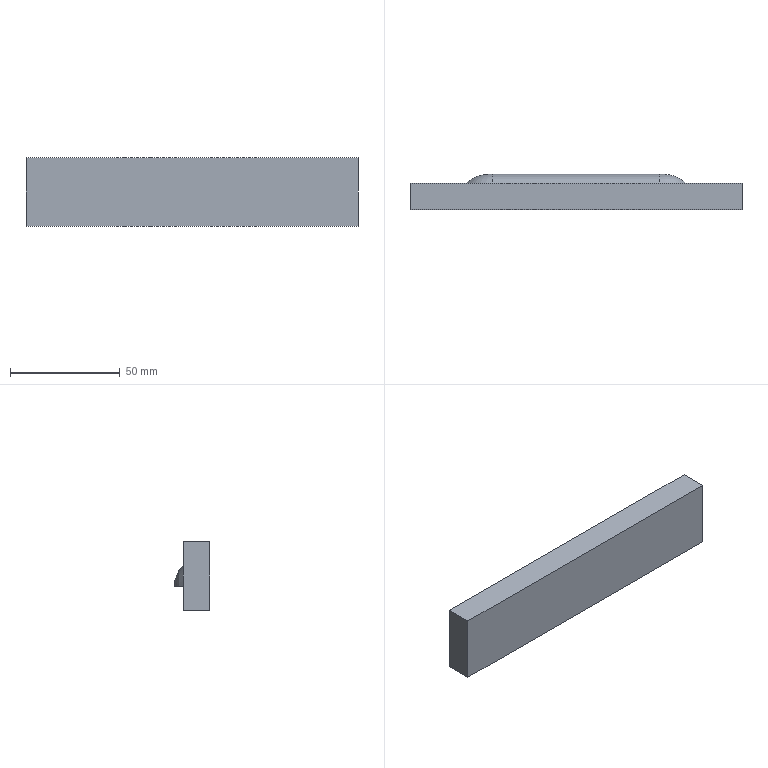Part | SolidWorks | features Fillet 2, Extrusion 1, FormToolCreator 1, ICE 1 | 1 solid | 10 faces | box 151.025 x 16 x 31.377 mm | volume 59353 mm3 | plane 7 | torus 2 | cylinder 1 | commonest cylinder face diameters 29 x1
STEP:
#1=CARTESIAN_POINT('',(75.513,12.,15.689));
#2=VERTEX_POINT('',#1);
#3=CARTESIAN_POINT('',(75.513,12.,-15.689));
#4=VERTEX_POINT('',#3);
#5=CARTESIAN_POINT('',(75.513,12.,-15.689));
#6=DIRECTION('',(0.,0.,-1.));
#7=VECTOR('',#6,1000.);
#8=LINE('',#5,#7);
#9=EDGE_CURVE('',#2,#4,#8,.T.);
#10=ORIENTED_EDGE('',*,*,#9,.T.);
#11=CARTESIAN_POINT('',(-75.513,12.,-15.689));
#12=VERTEX_POINT('',#11);
#13=CARTESIAN_POINT('',(-75.513,12.,-15.689));
#14=DIRECTION('',(-1.,0.,0.));
#15=VECTOR('',#14,1000.);
#16=LINE('',#13,#15);
#17=EDGE_CURVE('',#4,#12,#16,.T.);
#18=ORIENTED_EDGE('',*,*,#17,.T.);
#19=CARTESIAN_POINT('',(-75.513,12.,15.689));
#20=VERTEX_POINT('',#19);
#21=CARTESIAN_POINT('',(-75.513,12.,-15.689));
#22=DIRECTION('',(0.,0.,1.));
#23=VECTOR('',#22,1000.);
#24=LINE('',#21,#23);
#25=EDGE_CURVE('',#12,#20,#24,.T.);
#26=ORIENTED_EDGE('',*,*,#25,.T.);
#27=CARTESIAN_POINT('',(-75.513,12.,15.689));
#28=DIRECTION('',(1.,0.,0.));
#29=VECTOR('',#28,1000.);
#30=LINE('',#27,#29);
#31=EDGE_CURVE('',#20,#2,#30,.T.);
#32=ORIENTED_EDGE('',*,*,#31,.T.);
#33=EDGE_LOOP('',(#10,#18,#26,#32));
#34=FACE_OUTER_BOUND('',#33,.T.);
#35=CARTESIAN_POINT('',(50.,12.,-5.));
#36=VERTEX_POINT('',#35);
#37=CARTESIAN_POINT('',(-50.,12.,-5.));
#38=VERTEX_POINT('',#37);
#39=CARTESIAN_POINT('',(-50.,12.,-5.));
#40=DIRECTION('',(-1.,0.,0.));
#41=VECTOR('',#40,1000.);
#42=LINE('',#39,#41);
#43=EDGE_CURVE('',#36,#38,#42,.T.);
#44=ORIENTED_EDGE('',*,*,#43,.F.);
#45=CARTESIAN_POINT('',(38.168,12.,5.));
#46=VERTEX_POINT('',#45);
#47=CARTESIAN_POINT('',(38.168,12.,-7.));
#48=DIRECTION('',(0.,-1.,0.));
#49=DIRECTION('',(0.,0.,1.));
#50=AXIS2_PLACEMENT_3D('',#47,#48,#49);
#51=CIRCLE('',#50,12.);
#52=EDGE_CURVE('',#36,#46,#51,.T.);
#53=ORIENTED_EDGE('',*,*,#52,.T.);
#54=CARTESIAN_POINT('',(-38.168,12.,5.));
#55=VERTEX_POINT('',#54);
#56=CARTESIAN_POINT('',(-50.,12.,5.));
#57=DIRECTION('',(1.,0.,0.));
#58=VECTOR('',#57,1000.);
#59=LINE('',#56,#58);
#60=EDGE_CURVE('',#55,#46,#59,.T.);
#61=ORIENTED_EDGE('',*,*,#60,.F.);
#62=CARTESIAN_POINT('',(-38.168,12.,-7.));
#63=DIRECTION('',(0.,-1.,0.));
#64=DIRECTION('',(0.,0.,1.));
#65=AXIS2_PLACEMENT_3D('',#62,#63,#64);
#66=CIRCLE('',#65,12.);
#67=EDGE_CURVE('',#55,#38,#66,.T.);
#68=ORIENTED_EDGE('',*,*,#67,.T.);
#69=EDGE_LOOP('',(#44,#53,#61,#68));
#70=FACE_BOUND('',#69,.T.);
#71=CARTESIAN_POINT('',(0.,12.,0.));
#72=DIRECTION('',(0.,1.,0.));
#73=DIRECTION('',(0.,0.,1.));
#74=AXIS2_PLACEMENT_3D('',#71,#72,#73);
#75=PLANE('',#74);
#76=ADVANCED_FACE('',(#34,#70),#75,.T.);
#77=CARTESIAN_POINT('',(75.513,0.,15.689));
#78=VERTEX_POINT('',#77);
#79=CARTESIAN_POINT('',(75.513,0.,-15.689));
#80=VERTEX_POINT('',#79);
#81=CARTESIAN_POINT('',(75.513,0.,-15.689));
#82=DIRECTION('',(0.,0.,-1.));
#83=VECTOR('',#82,1000.);
#84=LINE('',#81,#83);
#85=EDGE_CURVE('',#78,#80,#84,.T.);
#86=ORIENTED_EDGE('',*,*,#85,.T.);
#87=CARTESIAN_POINT('',(75.513,12.,-15.689));
#88=DIRECTION('',(0.,-1.,0.));
#89=VECTOR('',#88,1000.);
#90=LINE('',#87,#89);
#91=EDGE_CURVE('',#4,#80,#90,.T.);
#92=ORIENTED_EDGE('',*,*,#91,.F.);
#93=ORIENTED_EDGE('',*,*,#9,.F.);
#94=CARTESIAN_POINT('',(75.513,12.,15.689));
#95=DIRECTION('',(0.,-1.,0.));
#96=VECTOR('',#95,1000.);
#97=LINE('',#94,#96);
#98=EDGE_CURVE('',#2,#78,#97,.T.);
#99=ORIENTED_EDGE('',*,*,#98,.T.);
#100=EDGE_LOOP('',(#86,#92,#93,#99));
#101=FACE_OUTER_BOUND('',#100,.T.);
#102=CARTESIAN_POINT('',(75.513,12.,-15.689));
#103=DIRECTION('',(-1.,0.,0.));
#104=DIRECTION('',(0.,0.,1.));
#105=AXIS2_PLACEMENT_3D('',#102,#103,#104);
#106=PLANE('',#105);
#107=ADVANCED_FACE('',(#101),#106,.F.);
#108=CARTESIAN_POINT('',(-75.513,0.,-15.689));
#109=VERTEX_POINT('',#108);
#110=CARTESIAN_POINT('',(-75.513,0.,-15.689));
#111=DIRECTION('',(-1.,0.,0.));
#112=VECTOR('',#111,1000.);
#113=LINE('',#110,#112);
#114=EDGE_CURVE('',#80,#109,#113,.T.);
#115=ORIENTED_EDGE('',*,*,#114,.T.);
#116=CARTESIAN_POINT('',(-75.513,12.,-15.689));
#117=DIRECTION('',(0.,-1.,0.));
#118=VECTOR('',#117,1000.);
#119=LINE('',#116,#118);
#120=EDGE_CURVE('',#12,#109,#119,.T.);
#121=ORIENTED_EDGE('',*,*,#120,.F.);
#122=ORIENTED_EDGE('',*,*,#17,.F.);
#123=ORIENTED_EDGE('',*,*,#91,.T.);
#124=EDGE_LOOP('',(#115,#121,#122,#123));
#125=FACE_OUTER_BOUND('',#124,.T.);
#126=CARTESIAN_POINT('',(-75.513,12.,-15.689));
#127=DIRECTION('',(0.,0.,1.));
#128=DIRECTION('',(1.,0.,0.));
#129=AXIS2_PLACEMENT_3D('',#126,#127,#128);
#130=PLANE('',#129);
#131=ADVANCED_FACE('',(#125),#130,.F.);
#132=CARTESIAN_POINT('',(-75.513,0.,15.689));
#133=VERTEX_POINT('',#132);
#134=CARTESIAN_POINT('',(-75.513,0.,-15.689));
#135=DIRECTION('',(0.,0.,1.));
#136=VECTOR('',#135,1000.);
#137=LINE('',#134,#136);
#138=EDGE_CURVE('',#109,#133,#137,.T.);
#139=ORIENTED_EDGE('',*,*,#138,.T.);
#140=CARTESIAN_POINT('',(-75.513,12.,15.689));
#141=DIRECTION('',(0.,-1.,0.));
#142=VECTOR('',#141,1000.);
#143=LINE('',#140,#142);
#144=EDGE_CURVE('',#20,#133,#143,.T.);
#145=ORIENTED_EDGE('',*,*,#144,.F.);
#146=ORIENTED_EDGE('',*,*,#25,.F.);
#147=ORIENTED_EDGE('',*,*,#120,.T.);
#148=EDGE_LOOP('',(#139,#145,#146,#147));
#149=FACE_OUTER_BOUND('',#148,.T.);
#150=CARTESIAN_POINT('',(-75.513,12.,-15.689));
#151=DIRECTION('',(1.,0.,0.));
#152=DIRECTION('',(0.,0.,-1.));
#153=AXIS2_PLACEMENT_3D('',#150,#151,#152);
#154=PLANE('',#153);
#155=ADVANCED_FACE('',(#149),#154,.F.);
#156=CARTESIAN_POINT('',(-75.513,0.,15.689));
#157=DIRECTION('',(1.,0.,0.));
#158=VECTOR('',#157,1000.);
#159=LINE('',#156,#158);
#160=EDGE_CURVE('',#133,#78,#159,.T.);
#161=ORIENTED_EDGE('',*,*,#160,.T.);
#162=ORIENTED_EDGE('',*,*,#98,.F.);
#163=ORIENTED_EDGE('',*,*,#31,.F.);
#164=ORIENTED_EDGE('',*,*,#144,.T.);
#165=EDGE_LOOP('',(#161,#162,#163,#164));
#166=FACE_OUTER_BOUND('',#165,.T.);
#167=CARTESIAN_POINT('',(-75.513,12.,15.689));
#168=DIRECTION('',(0.,0.,-1.));
#169=DIRECTION('',(-1.,0.,0.));
#170=AXIS2_PLACEMENT_3D('',#167,#168,#169);
#171=PLANE('',#170);
#172=ADVANCED_FACE('',(#166),#171,.F.);
#173=ORIENTED_EDGE('',*,*,#85,.F.);
#174=ORIENTED_EDGE('',*,*,#160,.F.);
#175=ORIENTED_EDGE('',*,*,#138,.F.);
#176=ORIENTED_EDGE('',*,*,#114,.F.);
#177=EDGE_LOOP('',(#173,#174,#175,#176));
#178=FACE_OUTER_BOUND('',#177,.T.);
#179=CARTESIAN_POINT('',(0.,0.,0.));
#180=DIRECTION('',(0.,1.,0.));
#181=DIRECTION('',(0.,0.,1.));
#182=AXIS2_PLACEMENT_3D('',#179,#180,#181);
#183=PLANE('',#182);
#184=ADVANCED_FACE('',(#178),#183,.F.);
#185=ORIENTED_EDGE('',*,*,#43,.T.);
#186=CARTESIAN_POINT('',(-38.168,16.,-5.));
#187=VERTEX_POINT('',#186);
#188=CARTESIAN_POINT('',(-50.,12.,-5.));
#189=CARTESIAN_POINT('',(-49.214,12.738,-5.));
#190=CARTESIAN_POINT('',(-48.36,13.376,-5.));
#191=CARTESIAN_POINT('',(-46.984,14.187,-5.));
#192=CARTESIAN_POINT('',(-46.509,14.433,-5.));
#193=CARTESIAN_POINT('',(-45.526,14.875,-5.));
#194=CARTESIAN_POINT('',(-45.026,15.067,-5.));
#195=CARTESIAN_POINT('',(-43.504,15.56,-5.));
#196=CARTESIAN_POINT('',(-42.461,15.775,-5.));
#197=CARTESIAN_POINT('',(-40.856,15.945,-5.));
#198=CARTESIAN_POINT('',(-40.318,15.976,-5.));
#199=CARTESIAN_POINT('',(-39.244,16.002,-5.));
#200=CARTESIAN_POINT('',(-38.706,16.,-5.));
#201=CARTESIAN_POINT('',(-38.168,16.,-5.));
#202=B_SPLINE_CURVE_WITH_KNOTS('',3,(#188,#189,#190,#191,#192,#193,#194,#195,#196,#197,#198,#199,#200,#201),.UNSPECIFIED.,.F.,.F.,(4,2,2,2,2,2,4),(0.,0.00319,0.004785,0.006381,0.009571,0.01117,0.01276),.UNSPECIFIED.);
#203=EDGE_CURVE('',#38,#187,#202,.T.);
#204=ORIENTED_EDGE('',*,*,#203,.T.);
#205=CARTESIAN_POINT('',(38.168,16.,-5.));
#206=VERTEX_POINT('',#205);
#207=CARTESIAN_POINT('',(-50.,16.,-5.));
#208=DIRECTION('',(-1.,0.,0.));
#209=VECTOR('',#208,1000.);
#210=LINE('',#207,#209);
#211=EDGE_CURVE('',#206,#187,#210,.T.);
#212=ORIENTED_EDGE('',*,*,#211,.F.);
#213=CARTESIAN_POINT('',(38.168,16.,-5.));
#214=CARTESIAN_POINT('',(38.707,16.,-5.));
#215=CARTESIAN_POINT('',(39.245,16.002,-5.));
#216=CARTESIAN_POINT('',(40.323,15.975,-5.));
#217=CARTESIAN_POINT('',(40.86,15.945,-5.));
#218=CARTESIAN_POINT('',(42.454,15.776,-5.));
#219=CARTESIAN_POINT('',(43.496,15.562,-5.));
#220=CARTESIAN_POINT('',(45.022,15.069,-5.));
#221=CARTESIAN_POINT('',(45.528,14.874,-5.));
#222=CARTESIAN_POINT('',(46.509,14.434,-5.));
#223=CARTESIAN_POINT('',(46.983,14.188,-5.));
#224=CARTESIAN_POINT('',(48.358,13.378,-5.));
#225=CARTESIAN_POINT('',(49.212,12.74,-5.));
#226=CARTESIAN_POINT('',(50.,12.,-5.));
#227=B_SPLINE_CURVE_WITH_KNOTS('',3,(#213,#214,#215,#216,#217,#218,#219,#220,#221,#222,#223,#224,#225,#226),.UNSPECIFIED.,.F.,.F.,(4,2,2,2,2,2,4),(0.,0.001616,0.003232,0.006465,0.008081,0.009697,0.01293),.UNSPECIFIED.);
#228=EDGE_CURVE('',#206,#36,#227,.T.);
#229=ORIENTED_EDGE('',*,*,#228,.T.);
#230=EDGE_LOOP('',(#185,#204,#212,#229));
#231=FACE_OUTER_BOUND('',#230,.T.);
#232=CARTESIAN_POINT('',(-50.,16.,-5.));
#233=DIRECTION('',(0.,0.,1.));
#234=DIRECTION('',(1.,0.,0.));
#235=AXIS2_PLACEMENT_3D('',#232,#233,#234);
#236=PLANE('',#235);
#237=ADVANCED_FACE('',(#231),#236,.F.);
#238=ORIENTED_EDGE('',*,*,#228,.F.);
#239=CARTESIAN_POINT('',(38.168,1.5,-5.));
#240=DIRECTION('',(-1.,0.,0.));
#241=DIRECTION('',(0.,-1.,0.));
#242=AXIS2_PLACEMENT_3D('',#239,#240,#241);
#243=CIRCLE('',#242,14.5);
#244=EDGE_CURVE('',#46,#206,#243,.T.);
#245=ORIENTED_EDGE('',*,*,#244,.F.);
#246=ORIENTED_EDGE('',*,*,#52,.F.);
#247=EDGE_LOOP('',(#238,#245,#246));
#248=FACE_OUTER_BOUND('',#247,.T.);
#249=CARTESIAN_POINT('',(38.168,1.5,-7.));
#250=DIRECTION('',(0.,-1.,0.));
#251=DIRECTION('',(0.,0.,-1.));
#252=AXIS2_PLACEMENT_3D('',#249,#250,#251);
#253=TOROIDAL_SURFACE('',#252,2.,14.5);
#254=ADVANCED_FACE('',(#248),#253,.T.);
#255=ORIENTED_EDGE('',*,*,#244,.T.);
#256=ORIENTED_EDGE('',*,*,#211,.T.);
#257=CARTESIAN_POINT('',(-38.168,1.5,-5.));
#258=DIRECTION('',(-1.,0.,0.));
#259=DIRECTION('',(0.,0.,1.));
#260=AXIS2_PLACEMENT_3D('',#257,#258,#259);
#261=CIRCLE('',#260,14.5);
#262=EDGE_CURVE('',#55,#187,#261,.T.);
#263=ORIENTED_EDGE('',*,*,#262,.F.);
#264=ORIENTED_EDGE('',*,*,#60,.T.);
#265=EDGE_LOOP('',(#255,#256,#263,#264));
#266=FACE_OUTER_BOUND('',#265,.T.);
#267=CARTESIAN_POINT('',(-50.,1.5,-5.));
#268=DIRECTION('',(1.,0.,0.));
#269=DIRECTION('',(0.,0.,-1.));
#270=AXIS2_PLACEMENT_3D('',#267,#268,#269);
#271=CYLINDRICAL_SURFACE('',#270,14.5);
#272=ADVANCED_FACE('',(#266),#271,.T.);
#273=ORIENTED_EDGE('',*,*,#203,.F.);
#274=ORIENTED_EDGE('',*,*,#67,.F.);
#275=ORIENTED_EDGE('',*,*,#262,.T.);
#276=EDGE_LOOP('',(#273,#274,#275));
#277=FACE_OUTER_BOUND('',#276,.T.);
#278=CARTESIAN_POINT('',(-38.168,1.5,-7.));
#279=DIRECTION('',(0.,-1.,0.));
#280=DIRECTION('',(0.,0.,-1.));
#281=AXIS2_PLACEMENT_3D('',#278,#279,#280);
#282=TOROIDAL_SURFACE('',#281,2.,14.5);
#283=ADVANCED_FACE('',(#277),#282,.T.);
#284=CLOSED_SHELL('',(#76,#107,#131,#155,#172,#184,#237,#254,#272,#283));
#285=MANIFOLD_SOLID_BREP('',#284);
#286=CARTESIAN_POINT('',(0.,0.,0.));
#287=DIRECTION('',(0.,0.,1.));
#288=DIRECTION('',(1.,0.,0.));
#289=AXIS2_PLACEMENT_3D('',#286,#287,#288);
#290=(LENGTH_UNIT()NAMED_UNIT(*)SI_UNIT(.MILLI.,.METRE.));
#291=UNCERTAINTY_MEASURE_WITH_UNIT(LENGTH_MEASURE(0.00001),#290,'','');
#292=(NAMED_UNIT(*)PLANE_ANGLE_UNIT()SI_UNIT($,.RADIAN.));
#293=(NAMED_UNIT(*)SI_UNIT($,.STERADIAN.)SOLID_ANGLE_UNIT());
#294=(GEOMETRIC_REPRESENTATION_CONTEXT(3)GLOBAL_UNCERTAINTY_ASSIGNED_CONTEXT((#291))GLOBAL_UNIT_ASSIGNED_CONTEXT((#290,#292,#293))REPRESENTATION_CONTEXT('',''));
#295=ADVANCED_BREP_SHAPE_REPRESENTATION('',(#285,#289),#294);